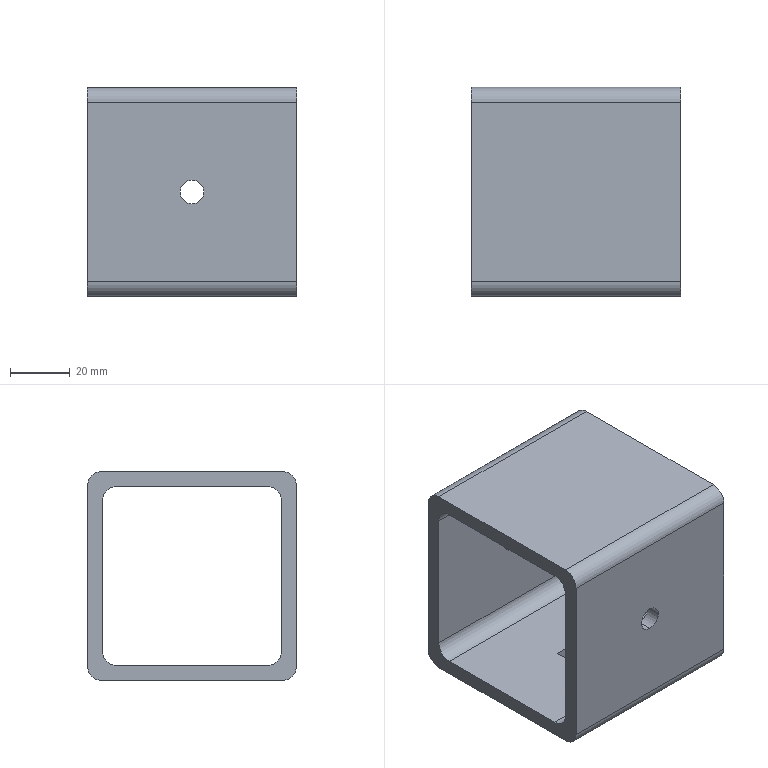Part | SolidWorks | features Cut 3, Extrusion 1, Fillet 1 | 1 solid | 26 faces | box 70 x 70 x 70 mm | volume 90163 mm3 | plane 14 | cylinder 12 | commonest cylinder face diameters 10 x8 8 x4
STEP:
#1=CARTESIAN_POINT('',(0.,-30.,39.));
#2=VERTEX_POINT('',#1);
#3=CARTESIAN_POINT('',(0.,-30.,31.));
#4=VERTEX_POINT('',#3);
#5=CARTESIAN_POINT('',(0.,-30.,35.));
#6=DIRECTION('',(0.,-1.,0.));
#7=DIRECTION('',(1.,0.,0.));
#8=AXIS2_PLACEMENT_3D('',#5,#6,#7);
#9=CIRCLE('',#8,4.);
#10=EDGE_CURVE('',#2,#4,#9,.T.);
#11=ORIENTED_EDGE('',*,*,#10,.F.);
#12=CARTESIAN_POINT('',(0.,-35.,39.));
#13=VERTEX_POINT('',#12);
#14=CARTESIAN_POINT('',(0.,87.,39.));
#15=DIRECTION('',(0.,-1.,0.));
#16=VECTOR('',#15,1000.);
#17=LINE('',#14,#16);
#18=EDGE_CURVE('',#2,#13,#17,.T.);
#19=ORIENTED_EDGE('',*,*,#18,.T.);
#20=CARTESIAN_POINT('',(0.,-35.,31.));
#21=VERTEX_POINT('',#20);
#22=CARTESIAN_POINT('',(0.,-35.,35.));
#23=DIRECTION('',(0.,-1.,0.));
#24=DIRECTION('',(0.,0.,-1.));
#25=AXIS2_PLACEMENT_3D('',#22,#23,#24);
#26=CIRCLE('',#25,4.);
#27=EDGE_CURVE('',#13,#21,#26,.T.);
#28=ORIENTED_EDGE('',*,*,#27,.T.);
#29=CARTESIAN_POINT('',(0.,87.,31.));
#30=DIRECTION('',(0.,-1.,0.));
#31=VECTOR('',#30,1000.);
#32=LINE('',#29,#31);
#33=EDGE_CURVE('',#4,#21,#32,.T.);
#34=ORIENTED_EDGE('',*,*,#33,.F.);
#35=EDGE_LOOP('',(#11,#19,#28,#34));
#36=FACE_OUTER_BOUND('',#35,.T.);
#37=CARTESIAN_POINT('',(0.,87.,35.));
#38=DIRECTION('',(0.,-1.,0.));
#39=DIRECTION('',(0.,0.,-1.));
#40=AXIS2_PLACEMENT_3D('',#37,#38,#39);
#41=CYLINDRICAL_SURFACE('',#40,4.);
#42=ADVANCED_FACE('',(#36),#41,.F.);
#43=CARTESIAN_POINT('',(0.,35.,39.));
#44=VERTEX_POINT('',#43);
#45=CARTESIAN_POINT('',(0.,35.,31.));
#46=VERTEX_POINT('',#45);
#47=CARTESIAN_POINT('',(0.,35.,35.));
#48=DIRECTION('',(0.,-1.,0.));
#49=DIRECTION('',(0.,0.,-1.));
#50=AXIS2_PLACEMENT_3D('',#47,#48,#49);
#51=CIRCLE('',#50,4.);
#52=EDGE_CURVE('',#44,#46,#51,.T.);
#53=ORIENTED_EDGE('',*,*,#52,.F.);
#54=CARTESIAN_POINT('',(0.,30.,39.));
#55=VERTEX_POINT('',#54);
#56=CARTESIAN_POINT('',(0.,87.,39.));
#57=DIRECTION('',(0.,-1.,0.));
#58=VECTOR('',#57,1000.);
#59=LINE('',#56,#58);
#60=EDGE_CURVE('',#44,#55,#59,.T.);
#61=ORIENTED_EDGE('',*,*,#60,.T.);
#62=CARTESIAN_POINT('',(0.,30.,31.));
#63=VERTEX_POINT('',#62);
#64=CARTESIAN_POINT('',(0.,30.,35.));
#65=DIRECTION('',(0.,1.,0.));
#66=DIRECTION('',(-1.,0.,0.));
#67=AXIS2_PLACEMENT_3D('',#64,#65,#66);
#68=CIRCLE('',#67,4.);
#69=EDGE_CURVE('',#63,#55,#68,.T.);
#70=ORIENTED_EDGE('',*,*,#69,.F.);
#71=CARTESIAN_POINT('',(0.,87.,31.));
#72=DIRECTION('',(0.,-1.,0.));
#73=VECTOR('',#72,1000.);
#74=LINE('',#71,#73);
#75=EDGE_CURVE('',#46,#63,#74,.T.);
#76=ORIENTED_EDGE('',*,*,#75,.F.);
#77=EDGE_LOOP('',(#53,#61,#70,#76));
#78=FACE_OUTER_BOUND('',#77,.T.);
#79=CARTESIAN_POINT('',(0.,87.,35.));
#80=DIRECTION('',(0.,-1.,0.));
#81=DIRECTION('',(0.,0.,-1.));
#82=AXIS2_PLACEMENT_3D('',#79,#80,#81);
#83=CYLINDRICAL_SURFACE('',#82,4.);
#84=ADVANCED_FACE('',(#78),#83,.F.);
#85=CARTESIAN_POINT('',(-35.,30.,10.));
#86=VERTEX_POINT('',#85);
#87=CARTESIAN_POINT('',(-35.,30.,60.));
#88=VERTEX_POINT('',#87);
#89=CARTESIAN_POINT('',(-35.,30.,70.));
#90=DIRECTION('',(0.,0.,1.));
#91=VECTOR('',#90,1000.);
#92=LINE('',#89,#91);
#93=EDGE_CURVE('',#86,#88,#92,.T.);
#94=ORIENTED_EDGE('',*,*,#93,.T.);
#95=CARTESIAN_POINT('',(-35.,25.,65.));
#96=VERTEX_POINT('',#95);
#97=CARTESIAN_POINT('',(-35.,25.,60.));
#98=DIRECTION('',(1.,0.,0.));
#99=DIRECTION('',(0.,1.,0.));
#100=AXIS2_PLACEMENT_3D('',#97,#98,#99);
#101=CIRCLE('',#100,5.);
#102=EDGE_CURVE('',#88,#96,#101,.T.);
#103=ORIENTED_EDGE('',*,*,#102,.T.);
#104=CARTESIAN_POINT('',(-35.,-25.,65.));
#105=VERTEX_POINT('',#104);
#106=CARTESIAN_POINT('',(-35.,35.,65.));
#107=DIRECTION('',(0.,-1.,0.));
#108=VECTOR('',#107,1000.);
#109=LINE('',#106,#108);
#110=EDGE_CURVE('',#96,#105,#109,.T.);
#111=ORIENTED_EDGE('',*,*,#110,.T.);
#112=CARTESIAN_POINT('',(-35.,-30.,60.));
#113=VERTEX_POINT('',#112);
#114=CARTESIAN_POINT('',(-35.,-25.,60.));
#115=DIRECTION('',(1.,0.,0.));
#116=DIRECTION('',(0.,1.,0.));
#117=AXIS2_PLACEMENT_3D('',#114,#115,#116);
#118=CIRCLE('',#117,5.);
#119=EDGE_CURVE('',#105,#113,#118,.T.);
#120=ORIENTED_EDGE('',*,*,#119,.T.);
#121=CARTESIAN_POINT('',(-35.,-30.,10.));
#122=VERTEX_POINT('',#121);
#123=CARTESIAN_POINT('',(-35.,-30.,70.));
#124=DIRECTION('',(0.,0.,-1.));
#125=VECTOR('',#124,1000.);
#126=LINE('',#123,#125);
#127=EDGE_CURVE('',#113,#122,#126,.T.);
#128=ORIENTED_EDGE('',*,*,#127,.T.);
#129=CARTESIAN_POINT('',(-35.,-25.,5.));
#130=VERTEX_POINT('',#129);
#131=CARTESIAN_POINT('',(-35.,-25.,10.));
#132=DIRECTION('',(1.,0.,0.));
#133=DIRECTION('',(0.,1.,0.));
#134=AXIS2_PLACEMENT_3D('',#131,#132,#133);
#135=CIRCLE('',#134,5.);
#136=EDGE_CURVE('',#122,#130,#135,.T.);
#137=ORIENTED_EDGE('',*,*,#136,.T.);
#138=CARTESIAN_POINT('',(-35.,25.,5.));
#139=VERTEX_POINT('',#138);
#140=CARTESIAN_POINT('',(-35.,35.,5.));
#141=DIRECTION('',(0.,1.,0.));
#142=VECTOR('',#141,1000.);
#143=LINE('',#140,#142);
#144=EDGE_CURVE('',#130,#139,#143,.T.);
#145=ORIENTED_EDGE('',*,*,#144,.T.);
#146=CARTESIAN_POINT('',(-35.,25.,10.));
#147=DIRECTION('',(1.,0.,0.));
#148=DIRECTION('',(0.,1.,0.));
#149=AXIS2_PLACEMENT_3D('',#146,#147,#148);
#150=CIRCLE('',#149,5.);
#151=EDGE_CURVE('',#139,#86,#150,.T.);
#152=ORIENTED_EDGE('',*,*,#151,.T.);
#153=EDGE_LOOP('',(#94,#103,#111,#120,#128,#137,#145,#152));
#154=FACE_BOUND('',#153,.T.);
#155=CARTESIAN_POINT('',(-35.,30.,70.));
#156=VERTEX_POINT('',#155);
#157=CARTESIAN_POINT('',(-35.,-30.,70.));
#158=VERTEX_POINT('',#157);
#159=CARTESIAN_POINT('',(-35.,35.,70.));
#160=DIRECTION('',(0.,-1.,0.));
#161=VECTOR('',#160,1000.);
#162=LINE('',#159,#161);
#163=EDGE_CURVE('',#156,#158,#162,.T.);
#164=ORIENTED_EDGE('',*,*,#163,.F.);
#165=CARTESIAN_POINT('',(-35.,35.,65.));
#166=VERTEX_POINT('',#165);
#167=CARTESIAN_POINT('',(-35.,30.,65.));
#168=DIRECTION('',(-1.,0.,0.));
#169=DIRECTION('',(0.,1.,0.));
#170=AXIS2_PLACEMENT_3D('',#167,#168,#169);
#171=CIRCLE('',#170,5.);
#172=EDGE_CURVE('',#156,#166,#171,.T.);
#173=ORIENTED_EDGE('',*,*,#172,.T.);
#174=CARTESIAN_POINT('',(-35.,35.,5.));
#175=VERTEX_POINT('',#174);
#176=CARTESIAN_POINT('',(-35.,35.,70.));
#177=DIRECTION('',(0.,0.,-1.));
#178=VECTOR('',#177,1000.);
#179=LINE('',#176,#178);
#180=EDGE_CURVE('',#166,#175,#179,.T.);
#181=ORIENTED_EDGE('',*,*,#180,.T.);
#182=CARTESIAN_POINT('',(-35.,30.,0.));
#183=VERTEX_POINT('',#182);
#184=CARTESIAN_POINT('',(-35.,30.,5.));
#185=DIRECTION('',(-1.,0.,0.));
#186=DIRECTION('',(0.,1.,0.));
#187=AXIS2_PLACEMENT_3D('',#184,#185,#186);
#188=CIRCLE('',#187,5.);
#189=EDGE_CURVE('',#175,#183,#188,.T.);
#190=ORIENTED_EDGE('',*,*,#189,.T.);
#191=CARTESIAN_POINT('',(-35.,-30.,0.));
#192=VERTEX_POINT('',#191);
#193=CARTESIAN_POINT('',(-35.,35.,0.));
#194=DIRECTION('',(0.,-1.,0.));
#195=VECTOR('',#194,1000.);
#196=LINE('',#193,#195);
#197=EDGE_CURVE('',#183,#192,#196,.T.);
#198=ORIENTED_EDGE('',*,*,#197,.T.);
#199=CARTESIAN_POINT('',(-35.,-35.,5.));
#200=VERTEX_POINT('',#199);
#201=CARTESIAN_POINT('',(-35.,-30.,5.));
#202=DIRECTION('',(-1.,0.,0.));
#203=DIRECTION('',(0.,1.,0.));
#204=AXIS2_PLACEMENT_3D('',#201,#202,#203);
#205=CIRCLE('',#204,5.);
#206=EDGE_CURVE('',#192,#200,#205,.T.);
#207=ORIENTED_EDGE('',*,*,#206,.T.);
#208=CARTESIAN_POINT('',(-35.,-35.,65.));
#209=VERTEX_POINT('',#208);
#210=CARTESIAN_POINT('',(-35.,-35.,70.));
#211=DIRECTION('',(0.,0.,-1.));
#212=VECTOR('',#211,1000.);
#213=LINE('',#210,#212);
#214=EDGE_CURVE('',#209,#200,#213,.T.);
#215=ORIENTED_EDGE('',*,*,#214,.F.);
#216=CARTESIAN_POINT('',(-35.,-30.,65.));
#217=DIRECTION('',(-1.,0.,0.));
#218=DIRECTION('',(0.,1.,0.));
#219=AXIS2_PLACEMENT_3D('',#216,#217,#218);
#220=CIRCLE('',#219,5.);
#221=EDGE_CURVE('',#209,#158,#220,.T.);
#222=ORIENTED_EDGE('',*,*,#221,.T.);
#223=EDGE_LOOP('',(#164,#173,#181,#190,#198,#207,#215,#222));
#224=FACE_OUTER_BOUND('',#223,.T.);
#225=CARTESIAN_POINT('',(-35.,35.,70.));
#226=DIRECTION('',(1.,0.,0.));
#227=DIRECTION('',(0.,1.,0.));
#228=AXIS2_PLACEMENT_3D('',#225,#226,#227);
#229=PLANE('',#228);
#230=ADVANCED_FACE('',(#154,#224),#229,.F.);
#231=CARTESIAN_POINT('',(0.,-35.,35.));
#232=DIRECTION('',(0.,-1.,0.));
#233=DIRECTION('',(0.,0.,-1.));
#234=AXIS2_PLACEMENT_3D('',#231,#232,#233);
#235=CIRCLE('',#234,4.);
#236=EDGE_CURVE('',#21,#13,#235,.T.);
#237=ORIENTED_EDGE('',*,*,#236,.F.);
#238=ORIENTED_EDGE('',*,*,#27,.F.);
#239=EDGE_LOOP('',(#237,#238));
#240=FACE_BOUND('',#239,.T.);
#241=CARTESIAN_POINT('',(35.,-35.,65.));
#242=VERTEX_POINT('',#241);
#243=CARTESIAN_POINT('',(35.,-35.,5.));
#244=VERTEX_POINT('',#243);
#245=CARTESIAN_POINT('',(35.,-35.,70.));
#246=DIRECTION('',(0.,0.,-1.));
#247=VECTOR('',#246,1000.);
#248=LINE('',#245,#247);
#249=EDGE_CURVE('',#242,#244,#248,.T.);
#250=ORIENTED_EDGE('',*,*,#249,.F.);
#251=CARTESIAN_POINT('',(35.,-35.,65.));
#252=DIRECTION('',(-1.,0.,0.));
#253=VECTOR('',#252,1000.);
#254=LINE('',#251,#253);
#255=EDGE_CURVE('',#242,#209,#254,.T.);
#256=ORIENTED_EDGE('',*,*,#255,.T.);
#257=ORIENTED_EDGE('',*,*,#214,.T.);
#258=CARTESIAN_POINT('',(35.,-35.,5.));
#259=DIRECTION('',(1.,0.,0.));
#260=VECTOR('',#259,1000.);
#261=LINE('',#258,#260);
#262=EDGE_CURVE('',#200,#244,#261,.T.);
#263=ORIENTED_EDGE('',*,*,#262,.T.);
#264=EDGE_LOOP('',(#250,#256,#257,#263));
#265=FACE_OUTER_BOUND('',#264,.T.);
#266=CARTESIAN_POINT('',(35.,-35.,70.));
#267=DIRECTION('',(0.,1.,0.));
#268=DIRECTION('',(0.,0.,1.));
#269=AXIS2_PLACEMENT_3D('',#266,#267,#268);
#270=PLANE('',#269);
#271=ADVANCED_FACE('',(#240,#265),#270,.F.);
#272=CARTESIAN_POINT('',(35.,-25.,5.));
#273=VERTEX_POINT('',#272);
#274=CARTESIAN_POINT('',(35.,25.,5.));
#275=VERTEX_POINT('',#274);
#276=CARTESIAN_POINT('',(35.,-30.,5.));
#277=DIRECTION('',(0.,1.,0.));
#278=VECTOR('',#277,1000.);
#279=LINE('',#276,#278);
#280=EDGE_CURVE('',#273,#275,#279,.T.);
#281=ORIENTED_EDGE('',*,*,#280,.F.);
#282=CARTESIAN_POINT('',(35.,-30.,10.));
#283=VERTEX_POINT('',#282);
#284=CARTESIAN_POINT('',(35.,-25.,10.));
#285=DIRECTION('',(-1.,0.,0.));
#286=DIRECTION('',(0.,-1.,0.));
#287=AXIS2_PLACEMENT_3D('',#284,#285,#286);
#288=CIRCLE('',#287,5.);
#289=EDGE_CURVE('',#273,#283,#288,.T.);
#290=ORIENTED_EDGE('',*,*,#289,.T.);
#291=CARTESIAN_POINT('',(35.,-30.,60.));
#292=VERTEX_POINT('',#291);
#293=CARTESIAN_POINT('',(35.,-30.,65.));
#294=DIRECTION('',(0.,0.,-1.));
#295=VECTOR('',#294,1000.);
#296=LINE('',#293,#295);
#297=EDGE_CURVE('',#292,#283,#296,.T.);
#298=ORIENTED_EDGE('',*,*,#297,.F.);
#299=CARTESIAN_POINT('',(35.,-25.,65.));
#300=VERTEX_POINT('',#299);
#301=CARTESIAN_POINT('',(35.,-25.,60.));
#302=DIRECTION('',(-1.,0.,0.));
#303=DIRECTION('',(0.,-1.,0.));
#304=AXIS2_PLACEMENT_3D('',#301,#302,#303);
#305=CIRCLE('',#304,5.);
#306=EDGE_CURVE('',#292,#300,#305,.T.);
#307=ORIENTED_EDGE('',*,*,#306,.T.);
#308=CARTESIAN_POINT('',(35.,25.,65.));
#309=VERTEX_POINT('',#308);
#310=CARTESIAN_POINT('',(35.,30.,65.));
#311=DIRECTION('',(0.,-1.,0.));
#312=VECTOR('',#311,1000.);
#313=LINE('',#310,#312);
#314=EDGE_CURVE('',#309,#300,#313,.T.);
#315=ORIENTED_EDGE('',*,*,#314,.F.);
#316=CARTESIAN_POINT('',(35.,30.,60.));
#317=VERTEX_POINT('',#316);
#318=CARTESIAN_POINT('',(35.,25.,60.));
#319=DIRECTION('',(-1.,0.,0.));
#320=DIRECTION('',(0.,-1.,0.));
#321=AXIS2_PLACEMENT_3D('',#318,#319,#320);
#322=CIRCLE('',#321,5.);
#323=EDGE_CURVE('',#309,#317,#322,.T.);
#324=ORIENTED_EDGE('',*,*,#323,.T.);
#325=CARTESIAN_POINT('',(35.,30.,10.));
#326=VERTEX_POINT('',#325);
#327=CARTESIAN_POINT('',(35.,30.,5.));
#328=DIRECTION('',(0.,0.,1.));
#329=VECTOR('',#328,1000.);
#330=LINE('',#327,#329);
#331=EDGE_CURVE('',#326,#317,#330,.T.);
#332=ORIENTED_EDGE('',*,*,#331,.F.);
#333=CARTESIAN_POINT('',(35.,25.,10.));
#334=DIRECTION('',(-1.,0.,0.));
#335=DIRECTION('',(0.,-1.,0.));
#336=AXIS2_PLACEMENT_3D('',#333,#334,#335);
#337=CIRCLE('',#336,5.);
#338=EDGE_CURVE('',#326,#275,#337,.T.);
#339=ORIENTED_EDGE('',*,*,#338,.T.);
#340=EDGE_LOOP('',(#281,#290,#298,#307,#315,#324,#332,#339));
#341=FACE_BOUND('',#340,.T.);
#342=CARTESIAN_POINT('',(35.,35.,65.));
#343=VERTEX_POINT('',#342);
#344=CARTESIAN_POINT('',(35.,35.,5.));
#345=VERTEX_POINT('',#344);
#346=CARTESIAN_POINT('',(35.,35.,70.));
#347=DIRECTION('',(0.,0.,-1.));
#348=VECTOR('',#347,1000.);
#349=LINE('',#346,#348);
#350=EDGE_CURVE('',#343,#345,#349,.T.);
#351=ORIENTED_EDGE('',*,*,#350,.F.);
#352=CARTESIAN_POINT('',(35.,30.,70.));
#353=VERTEX_POINT('',#352);
#354=CARTESIAN_POINT('',(35.,30.,65.));
#355=DIRECTION('',(1.,0.,0.));
#356=DIRECTION('',(0.,-1.,0.));
#357=AXIS2_PLACEMENT_3D('',#354,#355,#356);
#358=CIRCLE('',#357,5.);
#359=EDGE_CURVE('',#343,#353,#358,.T.);
#360=ORIENTED_EDGE('',*,*,#359,.T.);
#361=CARTESIAN_POINT('',(35.,-30.,70.));
#362=VERTEX_POINT('',#361);
#363=CARTESIAN_POINT('',(35.,35.,70.));
#364=DIRECTION('',(0.,1.,0.));
#365=VECTOR('',#364,1000.);
#366=LINE('',#363,#365);
#367=EDGE_CURVE('',#362,#353,#366,.T.);
#368=ORIENTED_EDGE('',*,*,#367,.F.);
#369=CARTESIAN_POINT('',(35.,-30.,65.));
#370=DIRECTION('',(1.,0.,0.));
#371=DIRECTION('',(0.,-1.,0.));
#372=AXIS2_PLACEMENT_3D('',#369,#370,#371);
#373=CIRCLE('',#372,5.);
#374=EDGE_CURVE('',#362,#242,#373,.T.);
#375=ORIENTED_EDGE('',*,*,#374,.T.);
#376=ORIENTED_EDGE('',*,*,#249,.T.);
#377=CARTESIAN_POINT('',(35.,-30.,0.));
#378=VERTEX_POINT('',#377);
#379=CARTESIAN_POINT('',(35.,-30.,5.));
#380=DIRECTION('',(1.,0.,0.));
#381=DIRECTION('',(0.,-1.,0.));
#382=AXIS2_PLACEMENT_3D('',#379,#380,#381);
#383=CIRCLE('',#382,5.);
#384=EDGE_CURVE('',#244,#378,#383,.T.);
#385=ORIENTED_EDGE('',*,*,#384,.T.);
#386=CARTESIAN_POINT('',(35.,30.,0.));
#387=VERTEX_POINT('',#386);
#388=CARTESIAN_POINT('',(35.,35.,0.));
#389=DIRECTION('',(0.,1.,0.));
#390=VECTOR('',#389,1000.);
#391=LINE('',#388,#390);
#392=EDGE_CURVE('',#378,#387,#391,.T.);
#393=ORIENTED_EDGE('',*,*,#392,.T.);
#394=CARTESIAN_POINT('',(35.,30.,5.));
#395=DIRECTION('',(1.,0.,0.));
#396=DIRECTION('',(0.,-1.,0.));
#397=AXIS2_PLACEMENT_3D('',#394,#395,#396);
#398=CIRCLE('',#397,5.);
#399=EDGE_CURVE('',#387,#345,#398,.T.);
#400=ORIENTED_EDGE('',*,*,#399,.T.);
#401=EDGE_LOOP('',(#351,#360,#368,#375,#376,#385,#393,#400));
#402=FACE_OUTER_BOUND('',#401,.T.);
#403=CARTESIAN_POINT('',(35.,35.,70.));
#404=DIRECTION('',(-1.,0.,0.));
#405=DIRECTION('',(0.,-1.,0.));
#406=AXIS2_PLACEMENT_3D('',#403,#404,#405);
#407=PLANE('',#406);
#408=ADVANCED_FACE('',(#341,#402),#407,.F.);
#409=CARTESIAN_POINT('',(0.,35.,35.));
#410=DIRECTION('',(0.,-1.,0.));
#411=DIRECTION('',(0.,0.,-1.));
#412=AXIS2_PLACEMENT_3D('',#409,#410,#411);
#413=CIRCLE('',#412,4.);
#414=EDGE_CURVE('',#46,#44,#413,.T.);
#415=ORIENTED_EDGE('',*,*,#414,.T.);
#416=ORIENTED_EDGE('',*,*,#52,.T.);
#417=EDGE_LOOP('',(#415,#416));
#418=FACE_BOUND('',#417,.T.);
#419=ORIENTED_EDGE('',*,*,#180,.F.);
#420=CARTESIAN_POINT('',(35.,35.,65.));
#421=DIRECTION('',(1.,0.,0.));
#422=VECTOR('',#421,1000.);
#423=LINE('',#420,#422);
#424=EDGE_CURVE('',#166,#343,#423,.T.);
#425=ORIENTED_EDGE('',*,*,#424,.T.);
#426=ORIENTED_EDGE('',*,*,#350,.T.);
#427=CARTESIAN_POINT('',(-35.,35.,5.));
#428=DIRECTION('',(-1.,0.,0.));
#429=VECTOR('',#428,1000.);
#430=LINE('',#427,#429);
#431=EDGE_CURVE('',#345,#175,#430,.T.);
#432=ORIENTED_EDGE('',*,*,#431,.T.);
#433=EDGE_LOOP('',(#419,#425,#426,#432));
#434=FACE_OUTER_BOUND('',#433,.T.);
#435=CARTESIAN_POINT('',(35.,35.,70.));
#436=DIRECTION('',(0.,-1.,0.));
#437=DIRECTION('',(0.,0.,-1.));
#438=AXIS2_PLACEMENT_3D('',#435,#436,#437);
#439=PLANE('',#438);
#440=ADVANCED_FACE('',(#418,#434),#439,.F.);
#441=ORIENTED_EDGE('',*,*,#367,.T.);
#442=CARTESIAN_POINT('',(0.,30.,70.));
#443=DIRECTION('',(-1.,0.,0.));
#444=VECTOR('',#443,1000.);
#445=LINE('',#442,#444);
#446=EDGE_CURVE('',#353,#156,#445,.T.);
#447=ORIENTED_EDGE('',*,*,#446,.T.);
#448=ORIENTED_EDGE('',*,*,#163,.T.);
#449=CARTESIAN_POINT('',(0.,-30.,70.));
#450=DIRECTION('',(1.,0.,0.));
#451=VECTOR('',#450,1000.);
#452=LINE('',#449,#451);
#453=EDGE_CURVE('',#158,#362,#452,.T.);
#454=ORIENTED_EDGE('',*,*,#453,.T.);
#455=EDGE_LOOP('',(#441,#447,#448,#454));
#456=FACE_OUTER_BOUND('',#455,.T.);
#457=CARTESIAN_POINT('',(0.,0.,70.));
#458=DIRECTION('',(0.,0.,-1.));
#459=DIRECTION('',(-1.,0.,0.));
#460=AXIS2_PLACEMENT_3D('',#457,#458,#459);
#461=PLANE('',#460);
#462=ADVANCED_FACE('',(#456),#461,.F.);
#463=CARTESIAN_POINT('',(6.2,2.7,0.));
#464=VERTEX_POINT('',#463);
#465=CARTESIAN_POINT('',(6.2,-2.7,0.));
#466=VERTEX_POINT('',#465);
#467=CARTESIAN_POINT('',(6.2,2.7,0.));
#468=DIRECTION('',(0.,-1.,0.));
#469=VECTOR('',#468,1000.);
#470=LINE('',#467,#469);
#471=EDGE_CURVE('',#464,#466,#470,.T.);
#472=ORIENTED_EDGE('',*,*,#471,.F.);
#473=CARTESIAN_POINT('',(-6.2,2.7,0.));
#474=VERTEX_POINT('',#473);
#475=CARTESIAN_POINT('',(-6.2,2.7,0.));
#476=DIRECTION('',(1.,0.,0.));
#477=VECTOR('',#476,1000.);
#478=LINE('',#475,#477);
#479=EDGE_CURVE('',#474,#464,#478,.T.);
#480=ORIENTED_EDGE('',*,*,#479,.F.);
#481=CARTESIAN_POINT('',(-6.2,-2.7,0.));
#482=VERTEX_POINT('',#481);
#483=CARTESIAN_POINT('',(-6.2,2.7,0.));
#484=DIRECTION('',(0.,1.,0.));
#485=VECTOR('',#484,1000.);
#486=LINE('',#483,#485);
#487=EDGE_CURVE('',#482,#474,#486,.T.);
#488=ORIENTED_EDGE('',*,*,#487,.F.);
#489=CARTESIAN_POINT('',(-6.2,-2.7,0.));
#490=DIRECTION('',(-1.,0.,0.));
#491=VECTOR('',#490,1000.);
#492=LINE('',#489,#491);
#493=EDGE_CURVE('',#466,#482,#492,.T.);
#494=ORIENTED_EDGE('',*,*,#493,.F.);
#495=EDGE_LOOP('',(#472,#480,#488,#494));
#496=FACE_BOUND('',#495,.T.);
#497=ORIENTED_EDGE('',*,*,#197,.F.);
#498=CARTESIAN_POINT('',(35.,30.,0.));
#499=DIRECTION('',(1.,0.,0.));
#500=VECTOR('',#499,1000.);
#501=LINE('',#498,#500);
#502=EDGE_CURVE('',#183,#387,#501,.T.);
#503=ORIENTED_EDGE('',*,*,#502,.T.);
#504=ORIENTED_EDGE('',*,*,#392,.F.);
#505=CARTESIAN_POINT('',(-35.,-30.,0.));
#506=DIRECTION('',(-1.,0.,0.));
#507=VECTOR('',#506,1000.);
#508=LINE('',#505,#507);
#509=EDGE_CURVE('',#378,#192,#508,.T.);
#510=ORIENTED_EDGE('',*,*,#509,.T.);
#511=EDGE_LOOP('',(#497,#503,#504,#510));
#512=FACE_OUTER_BOUND('',#511,.T.);
#513=CARTESIAN_POINT('',(0.,0.,0.));
#514=DIRECTION('',(0.,0.,-1.));
#515=DIRECTION('',(-1.,0.,0.));
#516=AXIS2_PLACEMENT_3D('',#513,#514,#515);
#517=PLANE('',#516);
#518=ADVANCED_FACE('',(#496,#512),#517,.T.);
#519=CARTESIAN_POINT('',(0.,-30.,35.));
#520=DIRECTION('',(0.,-1.,0.));
#521=DIRECTION('',(1.,0.,0.));
#522=AXIS2_PLACEMENT_3D('',#519,#520,#521);
#523=CIRCLE('',#522,4.);
#524=EDGE_CURVE('',#4,#2,#523,.T.);
#525=ORIENTED_EDGE('',*,*,#524,.T.);
#526=ORIENTED_EDGE('',*,*,#10,.T.);
#527=EDGE_LOOP('',(#525,#526));
#528=FACE_BOUND('',#527,.T.);
#529=ORIENTED_EDGE('',*,*,#127,.F.);
#530=CARTESIAN_POINT('',(35.,-30.,60.));
#531=DIRECTION('',(1.,0.,0.));
#532=VECTOR('',#531,1000.);
#533=LINE('',#530,#532);
#534=EDGE_CURVE('',#113,#292,#533,.T.);
#535=ORIENTED_EDGE('',*,*,#534,.T.);
#536=ORIENTED_EDGE('',*,*,#297,.T.);
#537=CARTESIAN_POINT('',(-35.,-30.,10.));
#538=DIRECTION('',(-1.,0.,0.));
#539=VECTOR('',#538,1000.);
#540=LINE('',#537,#539);
#541=EDGE_CURVE('',#283,#122,#540,.T.);
#542=ORIENTED_EDGE('',*,*,#541,.T.);
#543=EDGE_LOOP('',(#529,#535,#536,#542));
#544=FACE_OUTER_BOUND('',#543,.T.);
#545=CARTESIAN_POINT('',(-69.,-30.,65.));
#546=DIRECTION('',(0.,-1.,0.));
#547=DIRECTION('',(1.,0.,0.));
#548=AXIS2_PLACEMENT_3D('',#545,#546,#547);
#549=PLANE('',#548);
#550=ADVANCED_FACE('',(#528,#544),#549,.F.);
#551=ORIENTED_EDGE('',*,*,#110,.F.);
#552=CARTESIAN_POINT('',(35.,25.,65.));
#553=DIRECTION('',(1.,0.,0.));
#554=VECTOR('',#553,1000.);
#555=LINE('',#552,#554);
#556=EDGE_CURVE('',#96,#309,#555,.T.);
#557=ORIENTED_EDGE('',*,*,#556,.T.);
#558=ORIENTED_EDGE('',*,*,#314,.T.);
#559=CARTESIAN_POINT('',(-35.,-25.,65.));
#560=DIRECTION('',(-1.,0.,0.));
#561=VECTOR('',#560,1000.);
#562=LINE('',#559,#561);
#563=EDGE_CURVE('',#300,#105,#562,.T.);
#564=ORIENTED_EDGE('',*,*,#563,.T.);
#565=EDGE_LOOP('',(#551,#557,#558,#564));
#566=FACE_OUTER_BOUND('',#565,.T.);
#567=CARTESIAN_POINT('',(-69.,30.,65.));
#568=DIRECTION('',(0.,0.,1.));
#569=DIRECTION('',(1.,0.,0.));
#570=AXIS2_PLACEMENT_3D('',#567,#568,#569);
#571=PLANE('',#570);
#572=ADVANCED_FACE('',(#566),#571,.F.);
#573=ORIENTED_EDGE('',*,*,#69,.T.);
#574=CARTESIAN_POINT('',(0.,30.,35.));
#575=DIRECTION('',(0.,1.,0.));
#576=DIRECTION('',(-1.,0.,0.));
#577=AXIS2_PLACEMENT_3D('',#574,#575,#576);
#578=CIRCLE('',#577,4.);
#579=EDGE_CURVE('',#55,#63,#578,.T.);
#580=ORIENTED_EDGE('',*,*,#579,.T.);
#581=EDGE_LOOP('',(#573,#580));
#582=FACE_BOUND('',#581,.T.);
#583=ORIENTED_EDGE('',*,*,#331,.T.);
#584=CARTESIAN_POINT('',(-35.,30.,60.));
#585=DIRECTION('',(-1.,0.,0.));
#586=VECTOR('',#585,1000.);
#587=LINE('',#584,#586);
#588=EDGE_CURVE('',#317,#88,#587,.T.);
#589=ORIENTED_EDGE('',*,*,#588,.T.);
#590=ORIENTED_EDGE('',*,*,#93,.F.);
#591=CARTESIAN_POINT('',(35.,30.,10.));
#592=DIRECTION('',(1.,0.,0.));
#593=VECTOR('',#592,1000.);
#594=LINE('',#591,#593);
#595=EDGE_CURVE('',#86,#326,#594,.T.);
#596=ORIENTED_EDGE('',*,*,#595,.T.);
#597=EDGE_LOOP('',(#583,#589,#590,#596));
#598=FACE_OUTER_BOUND('',#597,.T.);
#599=CARTESIAN_POINT('',(-69.,30.,5.));
#600=DIRECTION('',(0.,1.,0.));
#601=DIRECTION('',(-1.,0.,0.));
#602=AXIS2_PLACEMENT_3D('',#599,#600,#601);
#603=PLANE('',#602);
#604=ADVANCED_FACE('',(#582,#598),#603,.F.);
#605=CARTESIAN_POINT('',(-6.2,2.7,5.));
#606=VERTEX_POINT('',#605);
#607=CARTESIAN_POINT('',(6.2,2.7,5.));
#608=VERTEX_POINT('',#607);
#609=CARTESIAN_POINT('',(-69.,2.7,5.));
#610=DIRECTION('',(1.,0.,0.));
#611=VECTOR('',#610,1000.);
#612=LINE('',#609,#611);
#613=EDGE_CURVE('',#606,#608,#612,.T.);
#614=ORIENTED_EDGE('',*,*,#613,.T.);
#615=CARTESIAN_POINT('',(6.2,-2.7,5.));
#616=VERTEX_POINT('',#615);
#617=CARTESIAN_POINT('',(6.2,-30.,5.));
#618=DIRECTION('',(0.,-1.,0.));
#619=VECTOR('',#618,1000.);
#620=LINE('',#617,#619);
#621=EDGE_CURVE('',#608,#616,#620,.T.);
#622=ORIENTED_EDGE('',*,*,#621,.T.);
#623=CARTESIAN_POINT('',(-6.2,-2.7,5.));
#624=VERTEX_POINT('',#623);
#625=CARTESIAN_POINT('',(-69.,-2.7,5.));
#626=DIRECTION('',(-1.,0.,0.));
#627=VECTOR('',#626,1000.);
#628=LINE('',#625,#627);
#629=EDGE_CURVE('',#616,#624,#628,.T.);
#630=ORIENTED_EDGE('',*,*,#629,.T.);
#631=CARTESIAN_POINT('',(-6.2,-30.,5.));
#632=DIRECTION('',(0.,1.,0.));
#633=VECTOR('',#632,1000.);
#634=LINE('',#631,#633);
#635=EDGE_CURVE('',#624,#606,#634,.T.);
#636=ORIENTED_EDGE('',*,*,#635,.T.);
#637=EDGE_LOOP('',(#614,#622,#630,#636));
#638=FACE_BOUND('',#637,.T.);
#639=ORIENTED_EDGE('',*,*,#144,.F.);
#640=CARTESIAN_POINT('',(35.,-25.,5.));
#641=DIRECTION('',(1.,0.,0.));
#642=VECTOR('',#641,1000.);
#643=LINE('',#640,#642);
#644=EDGE_CURVE('',#130,#273,#643,.T.);
#645=ORIENTED_EDGE('',*,*,#644,.T.);
#646=ORIENTED_EDGE('',*,*,#280,.T.);
#647=CARTESIAN_POINT('',(-35.,25.,5.));
#648=DIRECTION('',(-1.,0.,0.));
#649=VECTOR('',#648,1000.);
#650=LINE('',#647,#649);
#651=EDGE_CURVE('',#275,#139,#650,.T.);
#652=ORIENTED_EDGE('',*,*,#651,.T.);
#653=EDGE_LOOP('',(#639,#645,#646,#652));
#654=FACE_OUTER_BOUND('',#653,.T.);
#655=CARTESIAN_POINT('',(-69.,-30.,5.));
#656=DIRECTION('',(0.,0.,-1.));
#657=DIRECTION('',(-1.,0.,0.));
#658=AXIS2_PLACEMENT_3D('',#655,#656,#657);
#659=PLANE('',#658);
#660=ADVANCED_FACE('',(#638,#654),#659,.F.);
#661=CARTESIAN_POINT('',(6.2,2.7,10.));
#662=DIRECTION('',(0.,0.,-1.));
#663=VECTOR('',#662,1000.);
#664=LINE('',#661,#663);
#665=EDGE_CURVE('',#608,#464,#664,.T.);
#666=ORIENTED_EDGE('',*,*,#665,.T.);
#667=ORIENTED_EDGE('',*,*,#471,.T.);
#668=CARTESIAN_POINT('',(6.2,-2.7,10.));
#669=DIRECTION('',(0.,0.,-1.));
#670=VECTOR('',#669,1000.);
#671=LINE('',#668,#670);
#672=EDGE_CURVE('',#616,#466,#671,.T.);
#673=ORIENTED_EDGE('',*,*,#672,.F.);
#674=ORIENTED_EDGE('',*,*,#621,.F.);
#675=EDGE_LOOP('',(#666,#667,#673,#674));
#676=FACE_OUTER_BOUND('',#675,.T.);
#677=CARTESIAN_POINT('',(6.2,2.7,10.));
#678=DIRECTION('',(1.,0.,0.));
#679=DIRECTION('',(0.,0.,-1.));
#680=AXIS2_PLACEMENT_3D('',#677,#678,#679);
#681=PLANE('',#680);
#682=ADVANCED_FACE('',(#676),#681,.F.);
#683=CARTESIAN_POINT('',(-6.2,2.7,10.));
#684=DIRECTION('',(0.,0.,-1.));
#685=VECTOR('',#684,1000.);
#686=LINE('',#683,#685);
#687=EDGE_CURVE('',#606,#474,#686,.T.);
#688=ORIENTED_EDGE('',*,*,#687,.T.);
#689=ORIENTED_EDGE('',*,*,#479,.T.);
#690=ORIENTED_EDGE('',*,*,#665,.F.);
#691=ORIENTED_EDGE('',*,*,#613,.F.);
#692=EDGE_LOOP('',(#688,#689,#690,#691));
#693=FACE_OUTER_BOUND('',#692,.T.);
#694=CARTESIAN_POINT('',(-6.2,2.7,10.));
#695=DIRECTION('',(0.,1.,0.));
#696=DIRECTION('',(-1.,0.,0.));
#697=AXIS2_PLACEMENT_3D('',#694,#695,#696);
#698=PLANE('',#697);
#699=ADVANCED_FACE('',(#693),#698,.F.);
#700=CARTESIAN_POINT('',(-6.2,-2.7,10.));
#701=DIRECTION('',(0.,0.,-1.));
#702=VECTOR('',#701,1000.);
#703=LINE('',#700,#702);
#704=EDGE_CURVE('',#624,#482,#703,.T.);
#705=ORIENTED_EDGE('',*,*,#704,.T.);
#706=ORIENTED_EDGE('',*,*,#487,.T.);
#707=ORIENTED_EDGE('',*,*,#687,.F.);
#708=ORIENTED_EDGE('',*,*,#635,.F.);
#709=EDGE_LOOP('',(#705,#706,#707,#708));
#710=FACE_OUTER_BOUND('',#709,.T.);
#711=CARTESIAN_POINT('',(-6.2,2.7,10.));
#712=DIRECTION('',(-1.,0.,0.));
#713=DIRECTION('',(0.,0.,1.));
#714=AXIS2_PLACEMENT_3D('',#711,#712,#713);
#715=PLANE('',#714);
#716=ADVANCED_FACE('',(#710),#715,.F.);
#717=ORIENTED_EDGE('',*,*,#672,.T.);
#718=ORIENTED_EDGE('',*,*,#493,.T.);
#719=ORIENTED_EDGE('',*,*,#704,.F.);
#720=ORIENTED_EDGE('',*,*,#629,.F.);
#721=EDGE_LOOP('',(#717,#718,#719,#720));
#722=FACE_OUTER_BOUND('',#721,.T.);
#723=CARTESIAN_POINT('',(-6.2,-2.7,10.));
#724=DIRECTION('',(0.,-1.,0.));
#725=DIRECTION('',(1.,0.,0.));
#726=AXIS2_PLACEMENT_3D('',#723,#724,#725);
#727=PLANE('',#726);
#728=ADVANCED_FACE('',(#722),#727,.F.);
#729=ORIENTED_EDGE('',*,*,#60,.F.);
#730=ORIENTED_EDGE('',*,*,#414,.F.);
#731=ORIENTED_EDGE('',*,*,#75,.T.);
#732=ORIENTED_EDGE('',*,*,#579,.F.);
#733=EDGE_LOOP('',(#729,#730,#731,#732));
#734=FACE_OUTER_BOUND('',#733,.T.);
#735=CARTESIAN_POINT('',(0.,87.,35.));
#736=DIRECTION('',(0.,-1.,0.));
#737=DIRECTION('',(0.,0.,-1.));
#738=AXIS2_PLACEMENT_3D('',#735,#736,#737);
#739=CYLINDRICAL_SURFACE('',#738,4.);
#740=ADVANCED_FACE('',(#734),#739,.F.);
#741=ORIENTED_EDGE('',*,*,#18,.F.);
#742=ORIENTED_EDGE('',*,*,#524,.F.);
#743=ORIENTED_EDGE('',*,*,#33,.T.);
#744=ORIENTED_EDGE('',*,*,#236,.T.);
#745=EDGE_LOOP('',(#741,#742,#743,#744));
#746=FACE_OUTER_BOUND('',#745,.T.);
#747=CARTESIAN_POINT('',(0.,87.,35.));
#748=DIRECTION('',(0.,-1.,0.));
#749=DIRECTION('',(0.,0.,-1.));
#750=AXIS2_PLACEMENT_3D('',#747,#748,#749);
#751=CYLINDRICAL_SURFACE('',#750,4.);
#752=ADVANCED_FACE('',(#746),#751,.F.);
#753=ORIENTED_EDGE('',*,*,#359,.F.);
#754=ORIENTED_EDGE('',*,*,#424,.F.);
#755=ORIENTED_EDGE('',*,*,#172,.F.);
#756=ORIENTED_EDGE('',*,*,#446,.F.);
#757=EDGE_LOOP('',(#753,#754,#755,#756));
#758=FACE_OUTER_BOUND('',#757,.T.);
#759=CARTESIAN_POINT('',(0.,30.,65.));
#760=DIRECTION('',(-1.,0.,0.));
#761=DIRECTION('',(0.,0.,1.));
#762=AXIS2_PLACEMENT_3D('',#759,#760,#761);
#763=CYLINDRICAL_SURFACE('',#762,5.);
#764=ADVANCED_FACE('',(#758),#763,.T.);
#765=ORIENTED_EDGE('',*,*,#221,.F.);
#766=ORIENTED_EDGE('',*,*,#255,.F.);
#767=ORIENTED_EDGE('',*,*,#374,.F.);
#768=ORIENTED_EDGE('',*,*,#453,.F.);
#769=EDGE_LOOP('',(#765,#766,#767,#768));
#770=FACE_OUTER_BOUND('',#769,.T.);
#771=CARTESIAN_POINT('',(0.,-30.,65.));
#772=DIRECTION('',(1.,0.,0.));
#773=DIRECTION('',(0.,0.,-1.));
#774=AXIS2_PLACEMENT_3D('',#771,#772,#773);
#775=CYLINDRICAL_SURFACE('',#774,5.);
#776=ADVANCED_FACE('',(#770),#775,.T.);
#777=ORIENTED_EDGE('',*,*,#102,.F.);
#778=ORIENTED_EDGE('',*,*,#588,.F.);
#779=ORIENTED_EDGE('',*,*,#323,.F.);
#780=ORIENTED_EDGE('',*,*,#556,.F.);
#781=EDGE_LOOP('',(#777,#778,#779,#780));
#782=FACE_OUTER_BOUND('',#781,.T.);
#783=CARTESIAN_POINT('',(-69.,25.,60.));
#784=DIRECTION('',(-1.,0.,0.));
#785=DIRECTION('',(0.,-1.,0.));
#786=AXIS2_PLACEMENT_3D('',#783,#784,#785);
#787=CYLINDRICAL_SURFACE('',#786,5.);
#788=ADVANCED_FACE('',(#782),#787,.F.);
#789=ORIENTED_EDGE('',*,*,#119,.F.);
#790=ORIENTED_EDGE('',*,*,#563,.F.);
#791=ORIENTED_EDGE('',*,*,#306,.F.);
#792=ORIENTED_EDGE('',*,*,#534,.F.);
#793=EDGE_LOOP('',(#789,#790,#791,#792));
#794=FACE_OUTER_BOUND('',#793,.T.);
#795=CARTESIAN_POINT('',(-69.,-25.,60.));
#796=DIRECTION('',(-1.,0.,0.));
#797=DIRECTION('',(0.,-1.,0.));
#798=AXIS2_PLACEMENT_3D('',#795,#796,#797);
#799=CYLINDRICAL_SURFACE('',#798,5.);
#800=ADVANCED_FACE('',(#794),#799,.F.);
#801=ORIENTED_EDGE('',*,*,#136,.F.);
#802=ORIENTED_EDGE('',*,*,#541,.F.);
#803=ORIENTED_EDGE('',*,*,#289,.F.);
#804=ORIENTED_EDGE('',*,*,#644,.F.);
#805=EDGE_LOOP('',(#801,#802,#803,#804));
#806=FACE_OUTER_BOUND('',#805,.T.);
#807=CARTESIAN_POINT('',(-69.,-25.,10.));
#808=DIRECTION('',(-1.,0.,0.));
#809=DIRECTION('',(0.,-1.,0.));
#810=AXIS2_PLACEMENT_3D('',#807,#808,#809);
#811=CYLINDRICAL_SURFACE('',#810,5.);
#812=ADVANCED_FACE('',(#806),#811,.F.);
#813=ORIENTED_EDGE('',*,*,#151,.F.);
#814=ORIENTED_EDGE('',*,*,#651,.F.);
#815=ORIENTED_EDGE('',*,*,#338,.F.);
#816=ORIENTED_EDGE('',*,*,#595,.F.);
#817=EDGE_LOOP('',(#813,#814,#815,#816));
#818=FACE_OUTER_BOUND('',#817,.T.);
#819=CARTESIAN_POINT('',(-69.,25.,10.));
#820=DIRECTION('',(-1.,0.,0.));
#821=DIRECTION('',(0.,-1.,0.));
#822=AXIS2_PLACEMENT_3D('',#819,#820,#821);
#823=CYLINDRICAL_SURFACE('',#822,5.);
#824=ADVANCED_FACE('',(#818),#823,.F.);
#825=ORIENTED_EDGE('',*,*,#399,.F.);
#826=ORIENTED_EDGE('',*,*,#502,.F.);
#827=ORIENTED_EDGE('',*,*,#189,.F.);
#828=ORIENTED_EDGE('',*,*,#431,.F.);
#829=EDGE_LOOP('',(#825,#826,#827,#828));
#830=FACE_OUTER_BOUND('',#829,.T.);
#831=CARTESIAN_POINT('',(35.,30.,5.));
#832=DIRECTION('',(1.,0.,0.));
#833=DIRECTION('',(0.,0.,-1.));
#834=AXIS2_PLACEMENT_3D('',#831,#832,#833);
#835=CYLINDRICAL_SURFACE('',#834,5.);
#836=ADVANCED_FACE('',(#830),#835,.T.);
#837=ORIENTED_EDGE('',*,*,#206,.F.);
#838=ORIENTED_EDGE('',*,*,#509,.F.);
#839=ORIENTED_EDGE('',*,*,#384,.F.);
#840=ORIENTED_EDGE('',*,*,#262,.F.);
#841=EDGE_LOOP('',(#837,#838,#839,#840));
#842=FACE_OUTER_BOUND('',#841,.T.);
#843=CARTESIAN_POINT('',(35.,-30.,5.));
#844=DIRECTION('',(-1.,0.,0.));
#845=DIRECTION('',(0.,0.,1.));
#846=AXIS2_PLACEMENT_3D('',#843,#844,#845);
#847=CYLINDRICAL_SURFACE('',#846,5.);
#848=ADVANCED_FACE('',(#842),#847,.T.);
#849=CLOSED_SHELL('',(#42,#84,#230,#271,#408,#440,#462,#518,#550,#572,#604,#660,#682,#699,#716,#728,#740,#752,#764,#776,#788,#800,#812,#824,#836,#848));
#850=MANIFOLD_SOLID_BREP('',#849);
#851=CARTESIAN_POINT('',(0.,0.,0.));
#852=DIRECTION('',(0.,0.,1.));
#853=DIRECTION('',(1.,0.,0.));
#854=AXIS2_PLACEMENT_3D('',#851,#852,#853);
#855=(LENGTH_UNIT()NAMED_UNIT(*)SI_UNIT(.MILLI.,.METRE.));
#856=UNCERTAINTY_MEASURE_WITH_UNIT(LENGTH_MEASURE(0.00001),#855,'','');
#857=(NAMED_UNIT(*)PLANE_ANGLE_UNIT()SI_UNIT($,.RADIAN.));
#858=(NAMED_UNIT(*)SI_UNIT($,.STERADIAN.)SOLID_ANGLE_UNIT());
#859=(GEOMETRIC_REPRESENTATION_CONTEXT(3)GLOBAL_UNCERTAINTY_ASSIGNED_CONTEXT((#856))GLOBAL_UNIT_ASSIGNED_CONTEXT((#855,#857,#858))REPRESENTATION_CONTEXT('',''));
#860=ADVANCED_BREP_SHAPE_REPRESENTATION('',(#850,#854),#859);